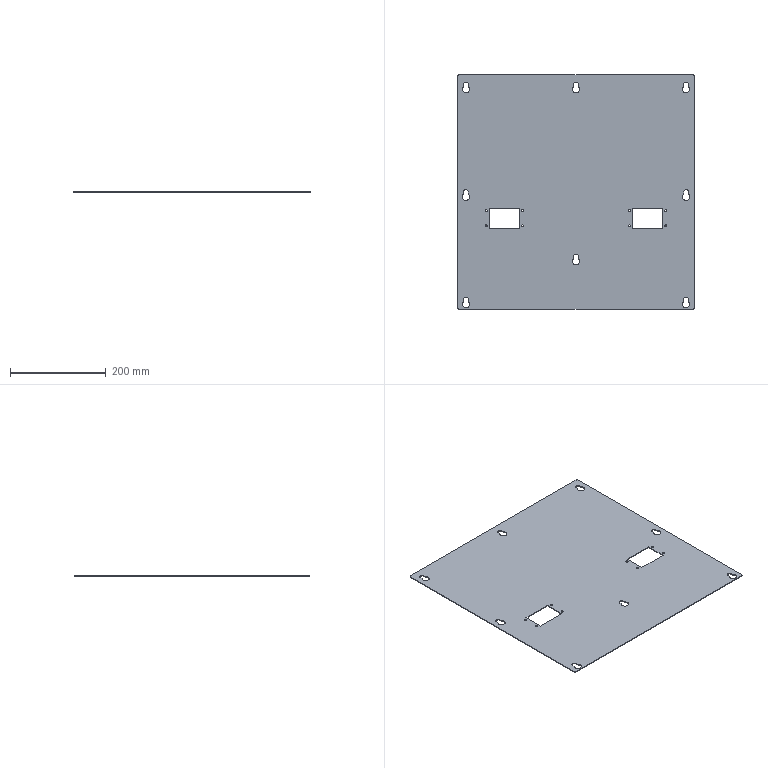Part | SolidWorks | features BaseBody 1 | 1 solid | 82 faces | box 496 x 490 x 1.5 mm | volume 353267 mm3 | cylinder 52 | plane 30 | commonest cylinder face diameters 15 x24 4.5 x16 10 x8 6 x4